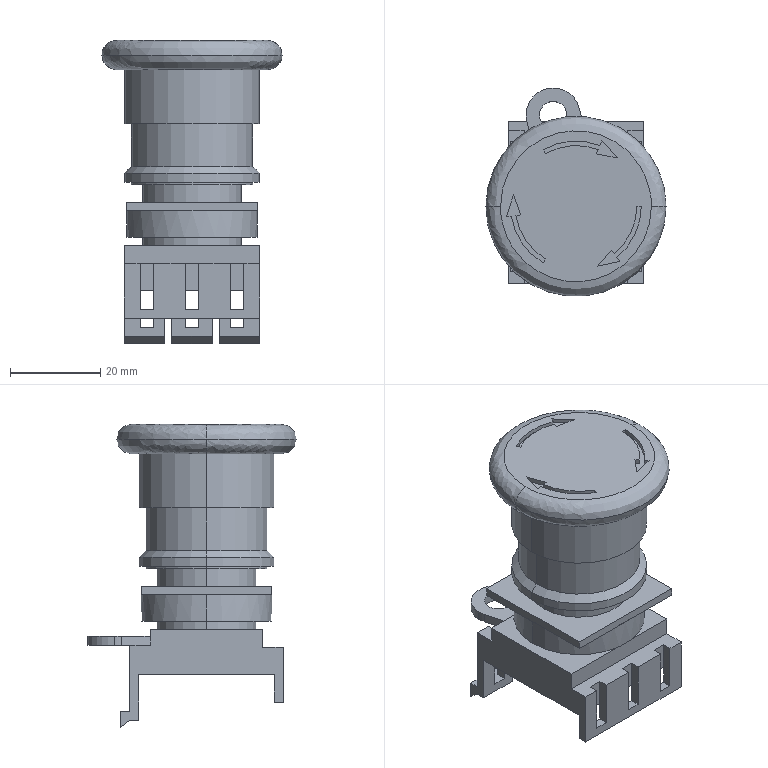Part | SolidWorks | features BaseBody 3 | 3 solids | 141 faces | box 40 x 46.376 x 67.3 mm | volume 38156 mm3 | plane 105 | cylinder 30 | spline 4 | cone 2 | commonest cylinder face diameters 27 x5 29 x5 20 x4 22 x4 30 x4 6 x2